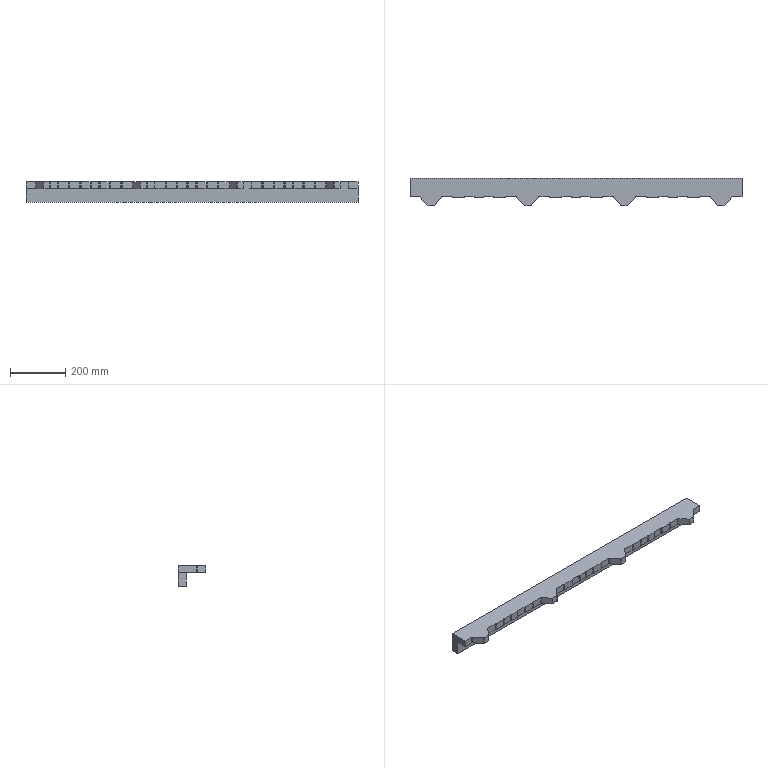Part | SolidWorks | features BaseBody 2 | 2 solids | 116 faces | box 1200 x 100 x 75 mm | volume 3996302 mm3 | plane 64 | cylinder 52 | commonest cylinder face diameters 6 x26 7 x26